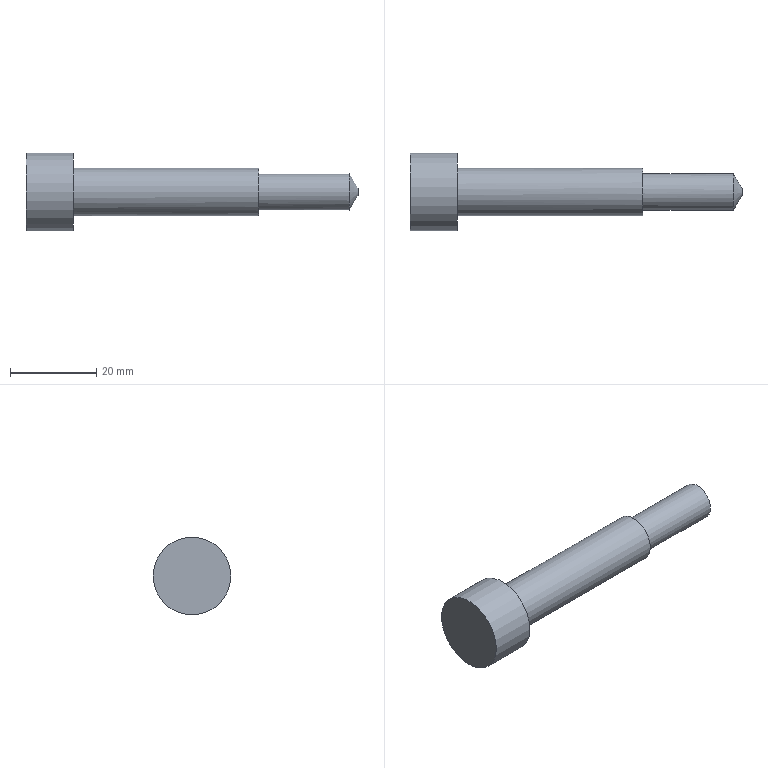Part | STEP file | solid 65 | 1 solid | 8 faces | box 77 x 18 x 18 mm | volume 8123 mm3 | plane 4 | cylinder 3 | cone 1 | commonest cylinder face diameters 8.5 x1 11 x1 18 x1